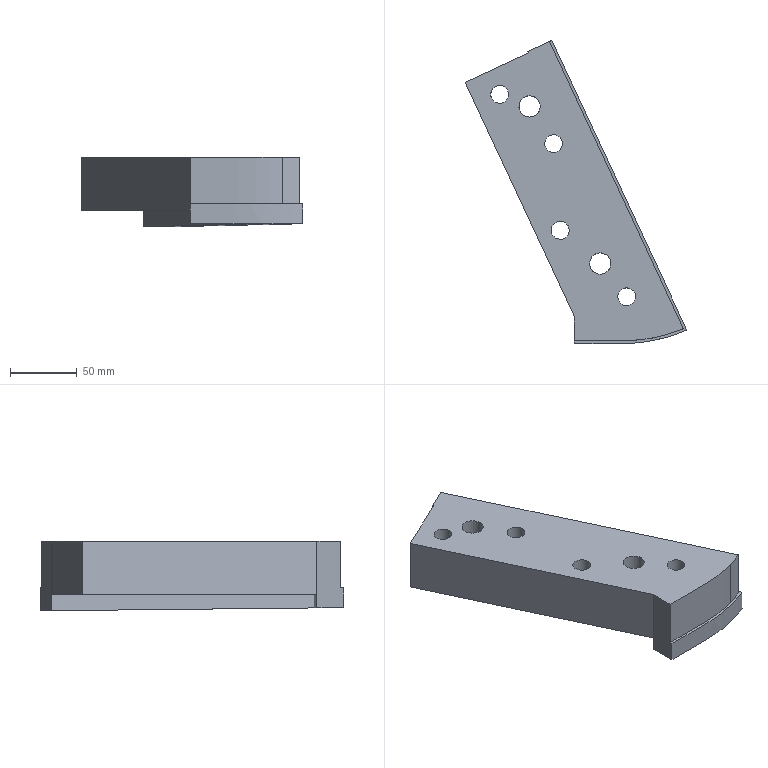Part | NX | features solid 2 | 1 solid | 32 faces | box 166.571 x 227.619 x 52.308 mm | volume 660539 mm3 | plane 17 | cylinder 10 | spline 5 | commonest cylinder face diameters 13.5 x4 19.5 x4 16 x2
STEP:
#1=CARTESIAN_POINT('',(214.067,-58.,43.));
#2=VERTEX_POINT('',#1);
#3=CARTESIAN_POINT('',(214.067,-58.,43.));
#4=VERTEX_POINT('',#3);
#5=CARTESIAN_POINT('',(192.036,-10.753,43.));
#6=DIRECTION('',(0.4226,-0.9063,0.));
#7=VECTOR('',#6,1000.);
#8=LINE('',#5,#7);
#9=EDGE_CURVE('',#2,#4,#8,.T.);
#10=ORIENTED_EDGE('',*,*,#9,.F.);
#11=CARTESIAN_POINT('',(214.067,-58.,8.));
#12=VERTEX_POINT('',#11);
#13=CARTESIAN_POINT('',(214.067,-58.,25.5));
#14=DIRECTION('',(0.,0.,-1.));
#15=VECTOR('',#14,1000.);
#16=LINE('',#13,#15);
#17=EDGE_CURVE('',#2,#12,#16,.T.);
#18=ORIENTED_EDGE('',*,*,#17,.T.);
#19=CARTESIAN_POINT('',(214.067,-58.,25.5));
#20=DIRECTION('',(0.,0.,-1.));
#21=VECTOR('',#20,1000.);
#22=LINE('',#19,#21);
#23=EDGE_CURVE('',#4,#12,#22,.T.);
#24=ORIENTED_EDGE('',*,*,#23,.F.);
#25=EDGE_LOOP('',(#10,#18,#24));
#26=FACE_BOUND('',#25,.T.);
#27=CARTESIAN_POINT('',(215.,-60.,-107.));
#28=DIRECTION('',(-0.9063,-0.4226,0.));
#29=DIRECTION('',(-0.4226,0.9063,0.));
#30=AXIS2_PLACEMENT_3D('',#27,#28,#29);
#31=PLANE('',#30);
#32=ADVANCED_FACE('',(#26),#31,.T.);
#33=CARTESIAN_POINT('',(170.586,159.137,-9.218));
#34=VERTEX_POINT('',#33);
#35=CARTESIAN_POINT('',(188.712,167.589,-9.308));
#36=VERTEX_POINT('',#35);
#37=CARTESIAN_POINT('',(155.822,152.253,-9.145));
#38=DIRECTION('',(-0.9063,-0.4226,0.004484));
#39=VECTOR('',#38,1000.);
#40=LINE('',#37,#39);
#41=EDGE_CURVE('',#34,#36,#40,.F.);
#42=ORIENTED_EDGE('',*,*,#41,.T.);
#43=CARTESIAN_POINT('',(290.127,-49.896,-7.));
#44=VERTEX_POINT('',#43);
#45=CARTESIAN_POINT('',(281.198,-30.747,-7.203));
#46=DIRECTION('',(-0.4226,0.9063,-0.009616));
#47=VECTOR('',#46,1000.);
#48=LINE('',#45,#47);
#49=EDGE_CURVE('',#36,#44,#48,.F.);
#50=ORIENTED_EDGE('',*,*,#49,.T.);
#51=CARTESIAN_POINT('',(205.676,-60.001,-6.893));
#52=VERTEX_POINT('',#51);
#53=CARTESIAN_POINT('',(205.676,-60.001,-6.893));
#54=CARTESIAN_POINT('',(212.807,-60.,-6.893));
#55=CARTESIAN_POINT('',(223.501,-59.952,-6.893));
#56=CARTESIAN_POINT('',(237.776,-60.073,-6.892));
#57=CARTESIAN_POINT('',(246.675,-59.905,-6.894));
#58=CARTESIAN_POINT('',(253.767,-59.465,-6.898));
#59=CARTESIAN_POINT('',(259.049,-58.73,-6.906));
#60=CARTESIAN_POINT('',(264.326,-57.938,-6.915));
#61=CARTESIAN_POINT('',(269.572,-56.804,-6.927));
#62=CARTESIAN_POINT('',(274.792,-55.406,-6.942));
#63=CARTESIAN_POINT('',(279.134,-54.082,-6.956));
#64=CARTESIAN_POINT('',(282.588,-52.985,-6.967));
#65=CARTESIAN_POINT('',(285.941,-51.62,-6.982));
#66=CARTESIAN_POINT('',(288.461,-50.608,-6.992));
#67=CARTESIAN_POINT('',(290.127,-49.896,-7.));
#68=B_SPLINE_CURVE_WITH_KNOTS('',3,(#53,#54,#55,#56,#57,#58,#59,#60,#61,#62,#63,#64,#65,#66,#67),.UNSPECIFIED.,.F.,.F.,(4,1,1,1,1,1,1,1,1,1,1,1,4),(-0.009286,0.01202,0.02268,0.03333,0.03866,0.04398,0.04931,0.05464,0.05996,0.06529,0.06795,0.07062,0.07594),.UNSPECIFIED.);
#69=EDGE_CURVE('',#52,#44,#68,.T.);
#70=ORIENTED_EDGE('',*,*,#69,.F.);
#71=CARTESIAN_POINT('',(205.675,-40.001,-7.105));
#72=VERTEX_POINT('',#71);
#73=CARTESIAN_POINT('',(205.675,-49.898,-7.));
#74=DIRECTION('',(0.00005303,-0.9999,0.01061));
#75=VECTOR('',#74,1000.);
#76=LINE('',#73,#75);
#77=EDGE_CURVE('',#72,#52,#76,.T.);
#78=ORIENTED_EDGE('',*,*,#77,.F.);
#79=CARTESIAN_POINT('',(205.674,-40.001,-7.105));
#80=VERTEX_POINT('',#79);
#81=CARTESIAN_POINT('',(215.618,-61.324,-6.879));
#82=DIRECTION('',(-0.4226,0.9063,-0.009616));
#83=VECTOR('',#82,1000.);
#84=LINE('',#81,#83);
#85=EDGE_CURVE('',#80,#72,#84,.F.);
#86=ORIENTED_EDGE('',*,*,#85,.F.);
#87=CARTESIAN_POINT('',(262.447,-37.86,-7.128));
#88=VERTEX_POINT('',#87);
#89=CARTESIAN_POINT('',(262.447,-37.86,-7.128));
#90=CARTESIAN_POINT('',(260.096,-38.349,-7.123));
#91=CARTESIAN_POINT('',(256.564,-38.895,-7.117));
#92=CARTESIAN_POINT('',(251.85,-39.528,-7.11));
#93=CARTESIAN_POINT('',(244.761,-40.001,-7.105));
#94=CARTESIAN_POINT('',(234.102,-40.028,-7.105));
#95=CARTESIAN_POINT('',(219.887,-39.989,-7.105));
#96=CARTESIAN_POINT('',(210.412,-40.,-7.105));
#97=CARTESIAN_POINT('',(205.674,-40.001,-7.105));
#98=B_SPLINE_CURVE_WITH_KNOTS('',3,(#89,#90,#91,#92,#93,#94,#95,#96,#97),.UNSPECIFIED.,.F.,.F.,(4,1,1,1,1,1,4),(0.,0.007102,0.01065,0.0142,0.02841,0.04261,0.05681),.UNSPECIFIED.);
#99=EDGE_CURVE('',#88,#80,#98,.T.);
#100=ORIENTED_EDGE('',*,*,#99,.F.);
#101=CARTESIAN_POINT('',(263.071,-39.199,-7.114));
#102=DIRECTION('',(-0.4226,0.9063,-0.009616));
#103=VECTOR('',#102,1000.);
#104=LINE('',#101,#103);
#105=EDGE_CURVE('',#34,#88,#104,.F.);
#106=ORIENTED_EDGE('',*,*,#105,.F.);
#107=EDGE_LOOP('',(#42,#50,#70,#78,#86,#100,#106));
#108=FACE_BOUND('',#107,.T.);
#109=CARTESIAN_POINT('',(240.127,-49.896,-7.));
#110=DIRECTION('',(0.,-0.01061,-0.9999));
#111=DIRECTION('',(0.,0.9999,-0.01061));
#112=AXIS2_PLACEMENT_3D('',#109,#110,#111);
#113=PLANE('',#112);
#114=ADVANCED_FACE('',(#108),#113,.T.);
#115=CARTESIAN_POINT('',(170.586,159.137,43.));
#116=VERTEX_POINT('',#115);
#117=CARTESIAN_POINT('',(171.008,158.231,43.));
#118=VERTEX_POINT('',#117);
#119=CARTESIAN_POINT('',(64.931,385.714,43.));
#120=DIRECTION('',(0.4226,-0.9063,0.));
#121=VECTOR('',#120,1000.);
#122=LINE('',#119,#121);
#123=EDGE_CURVE('',#116,#118,#122,.T.);
#124=ORIENTED_EDGE('',*,*,#123,.T.);
#125=CARTESIAN_POINT('',(123.556,136.103,43.));
#126=VERTEX_POINT('',#125);
#127=CARTESIAN_POINT('',(124.462,136.526,43.));
#128=DIRECTION('',(0.9063,0.4226,0.));
#129=VECTOR('',#128,1000.);
#130=LINE('',#127,#129);
#131=EDGE_CURVE('',#118,#126,#130,.F.);
#132=ORIENTED_EDGE('',*,*,#131,.T.);
#133=CARTESIAN_POINT('',(205.675,-40.001,43.));
#134=VERTEX_POINT('',#133);
#135=CARTESIAN_POINT('',(192.036,-10.753,43.));
#136=DIRECTION('',(0.4226,-0.9063,0.));
#137=VECTOR('',#136,1000.);
#138=LINE('',#135,#137);
#139=EDGE_CURVE('',#126,#134,#138,.T.);
#140=ORIENTED_EDGE('',*,*,#139,.T.);
#141=CARTESIAN_POINT('',(205.675,-58.001,43.));
#142=VERTEX_POINT('',#141);
#143=CARTESIAN_POINT('',(205.668,84.753,43.));
#144=DIRECTION('',(0.00005304,-1.,0.));
#145=VECTOR('',#144,1000.);
#146=LINE('',#143,#145);
#147=EDGE_CURVE('',#134,#142,#146,.T.);
#148=ORIENTED_EDGE('',*,*,#147,.T.);
#149=CARTESIAN_POINT('',(214.067,-58.,43.));
#150=CARTESIAN_POINT('',(211.27,-58.,43.));
#151=CARTESIAN_POINT('',(208.473,-58.,43.));
#152=CARTESIAN_POINT('',(205.675,-58.001,43.));
#153=B_SPLINE_CURVE_WITH_KNOTS('',3,(#149,#150,#151,#152),.UNSPECIFIED.,.F.,.F.,(4,4),(0.7754,0.7842),.UNSPECIFIED.);
#154=EDGE_CURVE('',#2,#142,#153,.T.);
#155=ORIENTED_EDGE('',*,*,#154,.F.);
#156=ORIENTED_EDGE('',*,*,#9,.T.);
#157=CARTESIAN_POINT('',(274.646,-53.334,43.));
#158=VERTEX_POINT('',#157);
#159=CARTESIAN_POINT('',(214.067,-58.,43.));
#160=CARTESIAN_POINT('',(219.163,-57.999,43.));
#161=CARTESIAN_POINT('',(229.355,-57.977,43.));
#162=CARTESIAN_POINT('',(242.09,-58.055,43.));
#163=CARTESIAN_POINT('',(252.284,-57.637,43.));
#164=CARTESIAN_POINT('',(259.807,-56.624,43.));
#165=CARTESIAN_POINT('',(267.291,-55.368,43.));
#166=CARTESIAN_POINT('',(272.199,-54.042,43.));
#167=CARTESIAN_POINT('',(274.646,-53.334,43.));
#168=B_SPLINE_CURVE_WITH_KNOTS('',3,(#159,#160,#161,#162,#163,#164,#165,#166,#167),.UNSPECIFIED.,.F.,.F.,(4,1,1,1,1,1,4),(-0.00294,0.01235,0.02763,0.03528,0.04292,0.05056,0.05821),.UNSPECIFIED.);
#169=EDGE_CURVE('',#4,#158,#168,.T.);
#170=ORIENTED_EDGE('',*,*,#169,.T.);
#171=CARTESIAN_POINT('',(274.646,-53.333,43.));
#172=VERTEX_POINT('',#171);
#173=CARTESIAN_POINT('',(262.155,89.442,43.));
#174=DIRECTION('',(0.08716,-0.9962,0.));
#175=VECTOR('',#174,1000.);
#176=LINE('',#173,#175);
#177=EDGE_CURVE('',#158,#172,#176,.F.);
#178=ORIENTED_EDGE('',*,*,#177,.T.);
#179=CARTESIAN_POINT('',(287.434,-48.854,43.));
#180=VERTEX_POINT('',#179);
#181=CARTESIAN_POINT('',(287.434,-48.854,43.));
#182=CARTESIAN_POINT('',(286.384,-49.285,43.));
#183=CARTESIAN_POINT('',(284.206,-50.176,43.));
#184=CARTESIAN_POINT('',(281.186,-51.367,43.));
#185=CARTESIAN_POINT('',(277.932,-52.345,43.));
#186=CARTESIAN_POINT('',(275.731,-53.015,43.));
#187=CARTESIAN_POINT('',(274.646,-53.333,43.));
#188=B_SPLINE_CURVE_WITH_KNOTS('',3,(#181,#182,#183,#184,#185,#186,#187),.UNSPECIFIED.,.F.,.F.,(4,1,1,1,4),(0.6964,0.7,0.7036,0.7072,0.7108),.UNSPECIFIED.);
#189=EDGE_CURVE('',#180,#172,#188,.T.);
#190=ORIENTED_EDGE('',*,*,#189,.F.);
#191=CARTESIAN_POINT('',(186.899,166.744,43.));
#192=VERTEX_POINT('',#191);
#193=CARTESIAN_POINT('',(81.245,393.321,43.));
#194=DIRECTION('',(-0.4226,0.9063,0.));
#195=VECTOR('',#194,1000.);
#196=LINE('',#193,#195);
#197=EDGE_CURVE('',#192,#180,#196,.F.);
#198=ORIENTED_EDGE('',*,*,#197,.F.);
#199=CARTESIAN_POINT('',(322.898,230.162,43.));
#200=DIRECTION('',(-0.9063,-0.4226,0.));
#201=VECTOR('',#200,1000.);
#202=LINE('',#199,#201);
#203=EDGE_CURVE('',#116,#192,#202,.F.);
#204=ORIENTED_EDGE('',*,*,#203,.F.);
#205=EDGE_LOOP('',(#124,#132,#140,#148,#155,#156,#170,#178,#190,#198,#204));
#206=FACE_BOUND('',#205,.T.);
#207=CARTESIAN_POINT('',(180.,118.,43.));
#208=VERTEX_POINT('',#207);
#209=CARTESIAN_POINT('',(172.,118.,43.));
#210=DIRECTION('',(0.,0.,1.));
#211=DIRECTION('',(1.,0.,0.));
#212=AXIS2_PLACEMENT_3D('',#209,#210,#211);
#213=CIRCLE('',#212,8.);
#214=EDGE_CURVE('',#208,#208,#213,.F.);
#215=ORIENTED_EDGE('',*,*,#214,.T.);
#216=EDGE_LOOP('',(#215));
#217=FACE_BOUND('',#216,.T.);
#218=CARTESIAN_POINT('',(233.,0.,43.));
#219=VERTEX_POINT('',#218);
#220=CARTESIAN_POINT('',(225.,0.,43.));
#221=DIRECTION('',(0.,0.,1.));
#222=DIRECTION('',(1.,0.,0.));
#223=AXIS2_PLACEMENT_3D('',#220,#221,#222);
#224=CIRCLE('',#223,8.);
#225=EDGE_CURVE('',#219,#219,#224,.F.);
#226=ORIENTED_EDGE('',*,*,#225,.T.);
#227=EDGE_LOOP('',(#226));
#228=FACE_BOUND('',#227,.T.);
#229=CARTESIAN_POINT('',(156.282,127.113,43.));
#230=VERTEX_POINT('',#229);
#231=CARTESIAN_POINT('',(149.532,127.113,43.));
#232=DIRECTION('',(0.,0.,1.));
#233=DIRECTION('',(1.,0.,0.));
#234=AXIS2_PLACEMENT_3D('',#231,#232,#233);
#235=CIRCLE('',#234,6.75);
#236=EDGE_CURVE('',#230,#230,#235,.F.);
#237=ORIENTED_EDGE('',*,*,#236,.T.);
#238=EDGE_LOOP('',(#237));
#239=FACE_BOUND('',#238,.T.);
#240=CARTESIAN_POINT('',(196.75,90.,43.));
#241=VERTEX_POINT('',#240);
#242=CARTESIAN_POINT('',(190.,90.,43.));
#243=DIRECTION('',(0.,0.,1.));
#244=DIRECTION('',(1.,0.,0.));
#245=AXIS2_PLACEMENT_3D('',#242,#243,#244);
#246=CIRCLE('',#245,6.75);
#247=EDGE_CURVE('',#241,#241,#246,.F.);
#248=ORIENTED_EDGE('',*,*,#247,.T.);
#249=EDGE_LOOP('',(#248));
#250=FACE_BOUND('',#249,.T.);
#251=CARTESIAN_POINT('',(201.75,25.,43.));
#252=VERTEX_POINT('',#251);
#253=CARTESIAN_POINT('',(195.,25.,43.));
#254=DIRECTION('',(0.,0.,1.));
#255=DIRECTION('',(1.,0.,0.));
#256=AXIS2_PLACEMENT_3D('',#253,#254,#255);
#257=CIRCLE('',#256,6.75);
#258=EDGE_CURVE('',#252,#252,#257,.F.);
#259=ORIENTED_EDGE('',*,*,#258,.T.);
#260=EDGE_LOOP('',(#259));
#261=FACE_BOUND('',#260,.T.);
#262=CARTESIAN_POINT('',(251.75,-25.,43.));
#263=VERTEX_POINT('',#262);
#264=CARTESIAN_POINT('',(245.,-25.,43.));
#265=DIRECTION('',(0.,0.,1.));
#266=DIRECTION('',(1.,0.,0.));
#267=AXIS2_PLACEMENT_3D('',#264,#265,#266);
#268=CIRCLE('',#267,6.75);
#269=EDGE_CURVE('',#263,#263,#268,.F.);
#270=ORIENTED_EDGE('',*,*,#269,.T.);
#271=EDGE_LOOP('',(#270));
#272=FACE_BOUND('',#271,.T.);
#273=CARTESIAN_POINT('',(383.563,100.064,43.));
#274=DIRECTION('',(0.,0.,-1.));
#275=DIRECTION('',(0.9962,0.08716,0.));
#276=AXIS2_PLACEMENT_3D('',#273,#274,#275);
#277=PLANE('',#276);
#278=ADVANCED_FACE('',(#206,#217,#228,#239,#250,#261,#272),#277,.F.);
#279=CARTESIAN_POINT('',(172.,110.,3.));
#280=VERTEX_POINT('',#279);
#281=CARTESIAN_POINT('',(172.,118.,3.));
#282=DIRECTION('',(0.,0.,-1.));
#283=DIRECTION('',(0.,-1.,0.));
#284=AXIS2_PLACEMENT_3D('',#281,#282,#283);
#285=CIRCLE('',#284,8.);
#286=EDGE_CURVE('',#280,#280,#285,.T.);
#287=ORIENTED_EDGE('',*,*,#286,.F.);
#288=EDGE_LOOP('',(#287));
#289=FACE_BOUND('',#288,.T.);
#290=CARTESIAN_POINT('',(225.,-8.,3.));
#291=VERTEX_POINT('',#290);
#292=CARTESIAN_POINT('',(225.,0.,3.));
#293=DIRECTION('',(0.,0.,-1.));
#294=DIRECTION('',(0.,-1.,0.));
#295=AXIS2_PLACEMENT_3D('',#292,#293,#294);
#296=CIRCLE('',#295,8.);
#297=EDGE_CURVE('',#291,#291,#296,.T.);
#298=ORIENTED_EDGE('',*,*,#297,.F.);
#299=EDGE_LOOP('',(#298));
#300=FACE_BOUND('',#299,.T.);
#301=CARTESIAN_POINT('',(149.532,117.363,3.));
#302=VERTEX_POINT('',#301);
#303=CARTESIAN_POINT('',(149.532,127.113,3.));
#304=DIRECTION('',(0.,0.,-1.));
#305=DIRECTION('',(0.,-1.,0.));
#306=AXIS2_PLACEMENT_3D('',#303,#304,#305);
#307=CIRCLE('',#306,9.75);
#308=EDGE_CURVE('',#302,#302,#307,.T.);
#309=ORIENTED_EDGE('',*,*,#308,.F.);
#310=EDGE_LOOP('',(#309));
#311=FACE_BOUND('',#310,.T.);
#312=CARTESIAN_POINT('',(190.,80.25,3.));
#313=VERTEX_POINT('',#312);
#314=CARTESIAN_POINT('',(190.,90.,3.));
#315=DIRECTION('',(0.,0.,-1.));
#316=DIRECTION('',(0.,-1.,0.));
#317=AXIS2_PLACEMENT_3D('',#314,#315,#316);
#318=CIRCLE('',#317,9.75);
#319=EDGE_CURVE('',#313,#313,#318,.T.);
#320=ORIENTED_EDGE('',*,*,#319,.F.);
#321=EDGE_LOOP('',(#320));
#322=FACE_BOUND('',#321,.T.);
#323=CARTESIAN_POINT('',(195.,15.25,3.));
#324=VERTEX_POINT('',#323);
#325=CARTESIAN_POINT('',(195.,25.,3.));
#326=DIRECTION('',(0.,0.,-1.));
#327=DIRECTION('',(0.,-1.,0.));
#328=AXIS2_PLACEMENT_3D('',#325,#326,#327);
#329=CIRCLE('',#328,9.75);
#330=EDGE_CURVE('',#324,#324,#329,.T.);
#331=ORIENTED_EDGE('',*,*,#330,.F.);
#332=EDGE_LOOP('',(#331));
#333=FACE_BOUND('',#332,.T.);
#334=CARTESIAN_POINT('',(245.,-34.75,3.));
#335=VERTEX_POINT('',#334);
#336=CARTESIAN_POINT('',(245.,-25.,3.));
#337=DIRECTION('',(0.,0.,-1.));
#338=DIRECTION('',(0.,-1.,0.));
#339=AXIS2_PLACEMENT_3D('',#336,#337,#338);
#340=CIRCLE('',#339,9.75);
#341=EDGE_CURVE('',#335,#335,#340,.T.);
#342=ORIENTED_EDGE('',*,*,#341,.F.);
#343=EDGE_LOOP('',(#342));
#344=FACE_BOUND('',#343,.T.);
#345=CARTESIAN_POINT('',(171.008,158.231,3.));
#346=VERTEX_POINT('',#345);
#347=CARTESIAN_POINT('',(123.556,136.103,3.));
#348=VERTEX_POINT('',#347);
#349=CARTESIAN_POINT('',(124.462,136.526,3.));
#350=DIRECTION('',(0.9063,0.4226,0.));
#351=VECTOR('',#350,1000.);
#352=LINE('',#349,#351);
#353=EDGE_CURVE('',#346,#348,#352,.F.);
#354=ORIENTED_EDGE('',*,*,#353,.F.);
#355=CARTESIAN_POINT('',(262.447,-37.86,3.));
#356=VERTEX_POINT('',#355);
#357=CARTESIAN_POINT('',(64.931,385.714,3.));
#358=DIRECTION('',(0.4226,-0.9063,0.));
#359=VECTOR('',#358,1000.);
#360=LINE('',#357,#359);
#361=EDGE_CURVE('',#346,#356,#360,.T.);
#362=ORIENTED_EDGE('',*,*,#361,.T.);
#363=CARTESIAN_POINT('',(205.674,-40.001,3.));
#364=VERTEX_POINT('',#363);
#365=CARTESIAN_POINT('',(262.447,-37.86,3.));
#366=CARTESIAN_POINT('',(260.12,-38.344,3.));
#367=CARTESIAN_POINT('',(256.612,-38.886,3.));
#368=CARTESIAN_POINT('',(251.926,-39.52,3.));
#369=CARTESIAN_POINT('',(244.85,-40.,3.));
#370=CARTESIAN_POINT('',(234.169,-40.029,3.));
#371=CARTESIAN_POINT('',(219.919,-39.989,3.));
#372=CARTESIAN_POINT('',(210.423,-40.,3.));
#373=CARTESIAN_POINT('',(205.674,-40.001,3.));
#374=B_SPLINE_CURVE_WITH_KNOTS('',3,(#365,#366,#367,#368,#369,#370,#371,#372,#373),.UNSPECIFIED.,.F.,.F.,(4,1,1,1,1,1,4),(0.07548,0.08262,0.08618,0.08975,0.104,0.1183,0.1325),.UNSPECIFIED.);
#375=EDGE_CURVE('',#364,#356,#374,.F.);
#376=ORIENTED_EDGE('',*,*,#375,.F.);
#377=CARTESIAN_POINT('',(204.661,-37.827,3.));
#378=DIRECTION('',(0.4226,-0.9063,0.));
#379=VECTOR('',#378,1000.);
#380=LINE('',#377,#379);
#381=EDGE_CURVE('',#364,#348,#380,.F.);
#382=ORIENTED_EDGE('',*,*,#381,.T.);
#383=EDGE_LOOP('',(#354,#362,#376,#382));
#384=FACE_BOUND('',#383,.T.);
#385=CARTESIAN_POINT('',(-60.069,387.73,3.));
#386=DIRECTION('',(0.,0.,-1.));
#387=DIRECTION('',(0.08716,-0.9962,0.));
#388=AXIS2_PLACEMENT_3D('',#385,#386,#387);
#389=PLANE('',#388);
#390=ADVANCED_FACE('',(#289,#300,#311,#322,#333,#344,#384),#389,.T.);
#391=CARTESIAN_POINT('',(188.712,167.589,8.));
#392=VERTEX_POINT('',#391);
#393=CARTESIAN_POINT('',(186.899,166.744,8.));
#394=VERTEX_POINT('',#393);
#395=CARTESIAN_POINT('',(85.717,119.562,8.));
#396=DIRECTION('',(0.9063,0.4226,0.));
#397=VECTOR('',#396,1000.);
#398=LINE('',#395,#397);
#399=EDGE_CURVE('',#392,#394,#398,.F.);
#400=ORIENTED_EDGE('',*,*,#399,.T.);
#401=CARTESIAN_POINT('',(287.434,-48.854,8.));
#402=VERTEX_POINT('',#401);
#403=CARTESIAN_POINT('',(81.245,393.321,8.));
#404=DIRECTION('',(-0.4226,0.9063,0.));
#405=VECTOR('',#404,1000.);
#406=LINE('',#403,#405);
#407=EDGE_CURVE('',#394,#402,#406,.F.);
#408=ORIENTED_EDGE('',*,*,#407,.T.);
#409=CARTESIAN_POINT('',(274.646,-53.333,8.));
#410=VERTEX_POINT('',#409);
#411=CARTESIAN_POINT('',(287.434,-48.854,8.));
#412=CARTESIAN_POINT('',(286.384,-49.285,8.));
#413=CARTESIAN_POINT('',(284.206,-50.176,8.));
#414=CARTESIAN_POINT('',(281.186,-51.367,8.));
#415=CARTESIAN_POINT('',(277.932,-52.345,8.));
#416=CARTESIAN_POINT('',(275.731,-53.015,8.));
#417=CARTESIAN_POINT('',(274.646,-53.333,8.));
#418=B_SPLINE_CURVE_WITH_KNOTS('',3,(#411,#412,#413,#414,#415,#416,#417),.UNSPECIFIED.,.F.,.F.,(4,1,1,1,4),(0.6964,0.7,0.7036,0.7072,0.7108),.UNSPECIFIED.);
#419=EDGE_CURVE('',#402,#410,#418,.T.);
#420=ORIENTED_EDGE('',*,*,#419,.T.);
#421=CARTESIAN_POINT('',(274.646,-53.334,8.));
#422=VERTEX_POINT('',#421);
#423=CARTESIAN_POINT('',(274.772,-54.771,8.));
#424=DIRECTION('',(-0.08716,0.9962,0.));
#425=VECTOR('',#424,1000.);
#426=LINE('',#423,#425);
#427=EDGE_CURVE('',#422,#410,#426,.T.);
#428=ORIENTED_EDGE('',*,*,#427,.F.);
#429=CARTESIAN_POINT('',(214.067,-58.,8.));
#430=CARTESIAN_POINT('',(219.163,-57.999,8.));
#431=CARTESIAN_POINT('',(229.355,-57.977,8.));
#432=CARTESIAN_POINT('',(242.089,-58.055,8.));
#433=CARTESIAN_POINT('',(252.284,-57.637,8.));
#434=CARTESIAN_POINT('',(259.807,-56.624,8.));
#435=CARTESIAN_POINT('',(267.292,-55.368,8.));
#436=CARTESIAN_POINT('',(272.2,-54.042,8.));
#437=CARTESIAN_POINT('',(274.646,-53.334,8.));
#438=B_SPLINE_CURVE_WITH_KNOTS('',3,(#429,#430,#431,#432,#433,#434,#435,#436,#437),.UNSPECIFIED.,.F.,.F.,(4,1,1,1,1,1,4),(-0.002765,0.01252,0.02781,0.03545,0.04309,0.05074,0.05838),.UNSPECIFIED.);
#439=EDGE_CURVE('',#12,#422,#438,.T.);
#440=ORIENTED_EDGE('',*,*,#439,.F.);
#441=CARTESIAN_POINT('',(205.675,-58.001,8.));
#442=VERTEX_POINT('',#441);
#443=CARTESIAN_POINT('',(214.067,-58.,8.));
#444=CARTESIAN_POINT('',(211.27,-58.,8.));
#445=CARTESIAN_POINT('',(208.473,-58.,8.));
#446=CARTESIAN_POINT('',(205.675,-58.001,8.));
#447=B_SPLINE_CURVE_WITH_KNOTS('',3,(#443,#444,#445,#446),.UNSPECIFIED.,.F.,.F.,(4,4),(0.7754,0.7842),.UNSPECIFIED.);
#448=EDGE_CURVE('',#12,#442,#447,.T.);
#449=ORIENTED_EDGE('',*,*,#448,.T.);
#450=CARTESIAN_POINT('',(205.676,-60.001,8.));
#451=VERTEX_POINT('',#450);
#452=CARTESIAN_POINT('',(205.65,429.974,8.));
#453=DIRECTION('',(-0.00005304,1.,0.));
#454=VECTOR('',#453,1000.);
#455=LINE('',#452,#454);
#456=EDGE_CURVE('',#442,#451,#455,.F.);
#457=ORIENTED_EDGE('',*,*,#456,.T.);
#458=CARTESIAN_POINT('',(215.,-60.,8.));
#459=VERTEX_POINT('',#458);
#460=CARTESIAN_POINT('',(205.676,-60.001,8.));
#461=CARTESIAN_POINT('',(206.425,-60.001,8.));
#462=CARTESIAN_POINT('',(207.882,-60.001,8.));
#463=CARTESIAN_POINT('',(211.055,-60.,8.));
#464=CARTESIAN_POINT('',(213.431,-60.,8.));
#465=CARTESIAN_POINT('',(215.,-60.,8.));
#466=B_SPLINE_CURVE_WITH_KNOTS('',3,(#460,#461,#462,#463,#464,#465),.UNSPECIFIED.,.F.,.F.,(4,1,1,4),(0.2156,0.2181,0.2206,0.2255),.UNSPECIFIED.);
#467=EDGE_CURVE('',#459,#451,#466,.F.);
#468=ORIENTED_EDGE('',*,*,#467,.F.);
#469=CARTESIAN_POINT('',(274.824,-55.364,8.));
#470=VERTEX_POINT('',#469);
#471=CARTESIAN_POINT('',(274.824,-55.364,8.));
#472=CARTESIAN_POINT('',(272.371,-56.074,8.));
#473=CARTESIAN_POINT('',(267.457,-57.375,8.));
#474=CARTESIAN_POINT('',(260.029,-58.61,8.));
#475=CARTESIAN_POINT('',(252.585,-59.618,8.));
#476=CARTESIAN_POINT('',(245.086,-59.927,8.));
#477=CARTESIAN_POINT('',(237.573,-60.058,8.));
#478=CARTESIAN_POINT('',(227.535,-59.965,8.));
#479=CARTESIAN_POINT('',(220.015,-59.999,8.));
#480=CARTESIAN_POINT('',(215.,-60.,8.));
#481=B_SPLINE_CURVE_WITH_KNOTS('',3,(#471,#472,#473,#474,#475,#476,#477,#478,#479,#480),.UNSPECIFIED.,.F.,.F.,(4,1,1,1,1,1,1,4),(0.,0.0075,0.015,0.0225,0.03,0.0375,0.045,0.06),.UNSPECIFIED.);
#482=EDGE_CURVE('',#470,#459,#481,.T.);
#483=ORIENTED_EDGE('',*,*,#482,.F.);
#484=CARTESIAN_POINT('',(290.127,-49.896,8.));
#485=VERTEX_POINT('',#484);
#486=CARTESIAN_POINT('',(274.824,-55.364,8.));
#487=CARTESIAN_POINT('',(275.15,-55.27,8.));
#488=CARTESIAN_POINT('',(275.64,-55.126,8.));
#489=CARTESIAN_POINT('',(276.722,-54.802,8.));
#490=CARTESIAN_POINT('',(277.734,-54.497,8.));
#491=CARTESIAN_POINT('',(278.338,-54.314,8.));
#492=CARTESIAN_POINT('',(278.669,-54.213,8.));
#493=CARTESIAN_POINT('',(279.265,-54.031,8.));
#494=CARTESIAN_POINT('',(279.745,-53.883,8.));
#495=CARTESIAN_POINT('',(280.187,-53.745,8.));
#496=CARTESIAN_POINT('',(280.814,-53.548,8.));
#497=CARTESIAN_POINT('',(281.532,-53.313,8.));
#498=CARTESIAN_POINT('',(282.084,-53.126,8.));
#499=CARTESIAN_POINT('',(282.731,-52.898,8.));
#500=CARTESIAN_POINT('',(283.309,-52.682,8.));
#501=CARTESIAN_POINT('',(283.991,-52.414,8.));
#502=CARTESIAN_POINT('',(284.387,-52.255,8.));
#503=CARTESIAN_POINT('',(284.936,-52.031,8.));
#504=CARTESIAN_POINT('',(285.292,-51.886,8.));
#505=CARTESIAN_POINT('',(285.642,-51.742,8.));
#506=CARTESIAN_POINT('',(285.81,-51.674,8.));
#507=CARTESIAN_POINT('',(286.171,-51.527,8.));
#508=CARTESIAN_POINT('',(286.882,-51.238,8.));
#509=CARTESIAN_POINT('',(287.218,-51.102,8.));
#510=CARTESIAN_POINT('',(287.366,-51.042,8.));
#511=CARTESIAN_POINT('',(287.365,-51.042,8.));
#512=CARTESIAN_POINT('',(287.562,-50.962,8.));
#513=CARTESIAN_POINT('',(287.858,-50.842,8.));
#514=CARTESIAN_POINT('',(288.274,-50.672,8.));
#515=CARTESIAN_POINT('',(288.732,-50.483,8.));
#516=CARTESIAN_POINT('',(289.243,-50.271,8.));
#517=CARTESIAN_POINT('',(289.804,-50.034,8.));
#518=CARTESIAN_POINT('',(290.127,-49.896,8.));
#519=B_SPLINE_CURVE_WITH_KNOTS('',3,(#486,#487,#488,#489,#490,#491,#492,#493,#494,#495,#496,#497,#498,#499,#500,#501,#502,#503,#504,#505,#506,#507,#508,#509,#510,#511,#512,#513,#514,#515,#516,#517,#518),.UNSPECIFIED.,.F.,.F.,(4,1,1,1,1,1,1,1,1,1,1,1,1,1,1,1,1,1,1,1,1,1,1,1,1,1,1,1,1,1,4),(0.2888,0.2898,0.2909,0.292,0.2925,0.293,0.2936,0.2941,0.2946,0.2952,0.2962,0.2967,0.2973,0.2983,0.2989,0.2994,0.2999,0.3005,0.3007,0.301,0.3015,0.3021,0.3023,0.3026,0.3027,0.3029,0.3031,0.3036,0.3042,0.3047,0.3058),.UNSPECIFIED.);
#520=EDGE_CURVE('',#485,#470,#519,.F.);
#521=ORIENTED_EDGE('',*,*,#520,.F.);
#522=CARTESIAN_POINT('',(178.495,189.499,8.));
#523=DIRECTION('',(-0.4226,0.9063,0.));
#524=VECTOR('',#523,1000.);
#525=LINE('',#522,#524);
#526=EDGE_CURVE('',#392,#485,#525,.F.);
#527=ORIENTED_EDGE('',*,*,#526,.F.);
#528=EDGE_LOOP('',(#400,#408,#420,#428,#440,#449,#457,#468,#483,#521,#527));
#529=FACE_BOUND('',#528,.T.);
#530=CARTESIAN_POINT('',(-40.145,389.473,8.));
#531=DIRECTION('',(0.,0.,1.));
#532=DIRECTION('',(0.08716,-0.9962,0.));
#533=AXIS2_PLACEMENT_3D('',#530,#531,#532);
#534=PLANE('',#533);
#535=ADVANCED_FACE('',(#529),#534,.T.);
#536=CARTESIAN_POINT('',(123.556,136.103,-107.));
#537=DIRECTION('',(0.,0.,1.));
#538=VECTOR('',#537,1000.);
#539=LINE('',#536,#538);
#540=EDGE_CURVE('',#348,#126,#539,.T.);
#541=ORIENTED_EDGE('',*,*,#540,.F.);
#542=ORIENTED_EDGE('',*,*,#381,.F.);
#543=CARTESIAN_POINT('',(205.674,-40.001,-4.5));
#544=DIRECTION('',(0.,0.,-1.));
#545=VECTOR('',#544,1000.);
#546=LINE('',#543,#545);
#547=EDGE_CURVE('',#364,#80,#546,.T.);
#548=ORIENTED_EDGE('',*,*,#547,.T.);
#549=ORIENTED_EDGE('',*,*,#85,.T.);
#550=CARTESIAN_POINT('',(205.675,-40.001,-107.));
#551=DIRECTION('',(0.,0.,1.));
#552=VECTOR('',#551,1000.);
#553=LINE('',#550,#552);
#554=EDGE_CURVE('',#72,#134,#553,.T.);
#555=ORIENTED_EDGE('',*,*,#554,.T.);
#556=ORIENTED_EDGE('',*,*,#139,.F.);
#557=EDGE_LOOP('',(#541,#542,#548,#549,#555,#556));
#558=FACE_BOUND('',#557,.T.);
#559=CARTESIAN_POINT('',(215.,-60.,-107.));
#560=DIRECTION('',(-0.9063,-0.4226,0.));
#561=DIRECTION('',(-0.4226,0.9063,0.));
#562=AXIS2_PLACEMENT_3D('',#559,#560,#561);
#563=PLANE('',#562);
#564=ADVANCED_FACE('',(#558),#563,.T.);
#565=CARTESIAN_POINT('',(188.712,167.589,-105.));
#566=DIRECTION('',(0.,0.,1.));
#567=VECTOR('',#566,1000.);
#568=LINE('',#565,#567);
#569=EDGE_CURVE('',#36,#392,#568,.T.);
#570=ORIENTED_EDGE('',*,*,#569,.T.);
#571=ORIENTED_EDGE('',*,*,#526,.T.);
#572=CARTESIAN_POINT('',(290.127,-49.896,0.5));
#573=DIRECTION('',(0.,0.,-1.));
#574=VECTOR('',#573,1000.);
#575=LINE('',#572,#574);
#576=EDGE_CURVE('',#485,#44,#575,.T.);
#577=ORIENTED_EDGE('',*,*,#576,.T.);
#578=ORIENTED_EDGE('',*,*,#49,.F.);
#579=EDGE_LOOP('',(#570,#571,#577,#578));
#580=FACE_BOUND('',#579,.T.);
#581=CARTESIAN_POINT('',(290.14,-49.924,-105.));
#582=DIRECTION('',(-0.9063,-0.4226,0.));
#583=DIRECTION('',(-0.4226,0.9063,0.));
#584=AXIS2_PLACEMENT_3D('',#581,#582,#583);
#585=PLANE('',#584);
#586=ADVANCED_FACE('',(#580),#585,.F.);
#587=ORIENTED_EDGE('',*,*,#105,.T.);
#588=CARTESIAN_POINT('',(262.447,-37.86,3.));
#589=DIRECTION('',(0.,0.,-1.));
#590=VECTOR('',#589,1000.);
#591=LINE('',#588,#590);
#592=EDGE_CURVE('',#88,#356,#591,.F.);
#593=ORIENTED_EDGE('',*,*,#592,.T.);
#594=ORIENTED_EDGE('',*,*,#361,.F.);
#595=CARTESIAN_POINT('',(171.008,158.231,3.));
#596=DIRECTION('',(0.,0.,-1.));
#597=VECTOR('',#596,1000.);
#598=LINE('',#595,#597);
#599=EDGE_CURVE('',#346,#118,#598,.F.);
#600=ORIENTED_EDGE('',*,*,#599,.T.);
#601=ORIENTED_EDGE('',*,*,#123,.F.);
#602=CARTESIAN_POINT('',(170.586,159.137,3.));
#603=DIRECTION('',(0.,0.,1.));
#604=VECTOR('',#603,1000.);
#605=LINE('',#602,#604);
#606=EDGE_CURVE('',#34,#116,#605,.T.);
#607=ORIENTED_EDGE('',*,*,#606,.F.);
#608=EDGE_LOOP('',(#587,#593,#594,#600,#601,#607));
#609=FACE_BOUND('',#608,.T.);
#610=CARTESIAN_POINT('',(64.931,385.714,3.));
#611=DIRECTION('',(-0.9063,-0.4226,0.));
#612=DIRECTION('',(-0.4226,0.9063,0.));
#613=AXIS2_PLACEMENT_3D('',#610,#611,#612);
#614=PLANE('',#613);
#615=ADVANCED_FACE('',(#609),#614,.T.);
#616=CARTESIAN_POINT('',(186.899,166.744,43.));
#617=DIRECTION('',(0.,0.,1.));
#618=VECTOR('',#617,1000.);
#619=LINE('',#616,#618);
#620=EDGE_CURVE('',#394,#192,#619,.T.);
#621=ORIENTED_EDGE('',*,*,#620,.T.);
#622=ORIENTED_EDGE('',*,*,#197,.T.);
#623=CARTESIAN_POINT('',(287.434,-48.854,25.5));
#624=DIRECTION('',(0.,0.,-1.));
#625=VECTOR('',#624,1000.);
#626=LINE('',#623,#625);
#627=EDGE_CURVE('',#180,#402,#626,.T.);
#628=ORIENTED_EDGE('',*,*,#627,.T.);
#629=ORIENTED_EDGE('',*,*,#407,.F.);
#630=EDGE_LOOP('',(#621,#622,#628,#629));
#631=FACE_BOUND('',#630,.T.);
#632=CARTESIAN_POINT('',(81.245,393.321,43.));
#633=DIRECTION('',(-0.9063,-0.4226,0.));
#634=DIRECTION('',(-0.4226,0.9063,0.));
#635=AXIS2_PLACEMENT_3D('',#632,#633,#634);
#636=PLANE('',#635);
#637=ADVANCED_FACE('',(#631),#636,.F.);
#638=CARTESIAN_POINT('',(274.646,-53.333,25.5));
#639=DIRECTION('',(0.,0.,-1.));
#640=VECTOR('',#639,1000.);
#641=LINE('',#638,#640);
#642=EDGE_CURVE('',#410,#172,#641,.F.);
#643=ORIENTED_EDGE('',*,*,#642,.T.);
#644=ORIENTED_EDGE('',*,*,#177,.F.);
#645=CARTESIAN_POINT('',(274.646,-53.334,33.));
#646=DIRECTION('',(0.,0.,-1.));
#647=VECTOR('',#646,1000.);
#648=LINE('',#645,#647);
#649=EDGE_CURVE('',#158,#422,#648,.T.);
#650=ORIENTED_EDGE('',*,*,#649,.T.);
#651=ORIENTED_EDGE('',*,*,#427,.T.);
#652=EDGE_LOOP('',(#643,#644,#650,#651));
#653=FACE_BOUND('',#652,.T.);
#654=CARTESIAN_POINT('',(274.772,-54.771,-5.));
#655=DIRECTION('',(-0.9962,-0.08716,0.));
#656=DIRECTION('',(0.,0.,-1.));
#657=AXIS2_PLACEMENT_3D('',#654,#655,#656);
#658=PLANE('',#657);
#659=ADVANCED_FACE('',(#653),#658,.F.);
#660=ORIENTED_EDGE('',*,*,#482,.T.);
#661=ORIENTED_EDGE('',*,*,#467,.T.);
#662=CARTESIAN_POINT('',(205.676,-60.001,0.5));
#663=DIRECTION('',(0.,0.,-1.));
#664=VECTOR('',#663,1000.);
#665=LINE('',#662,#664);
#666=EDGE_CURVE('',#451,#52,#665,.T.);
#667=ORIENTED_EDGE('',*,*,#666,.T.);
#668=ORIENTED_EDGE('',*,*,#69,.T.);
#669=ORIENTED_EDGE('',*,*,#576,.F.);
#670=ORIENTED_EDGE('',*,*,#520,.T.);
#671=EDGE_LOOP('',(#660,#661,#667,#668,#669,#670));
#672=FACE_BOUND('',#671,.T.);
#673=CARTESIAN_POINT('',(290.127,-49.896,8.));
#674=CARTESIAN_POINT('',(290.127,-49.896,-7.09));
#675=CARTESIAN_POINT('',(288.482,-50.599,8.));
#676=CARTESIAN_POINT('',(288.482,-50.599,-7.09));
#677=CARTESIAN_POINT('',(285.992,-51.597,8.));
#678=CARTESIAN_POINT('',(285.992,-51.597,-7.09));
#679=CARTESIAN_POINT('',(282.68,-52.951,8.));
#680=CARTESIAN_POINT('',(282.68,-52.951,-7.09));
#681=CARTESIAN_POINT('',(279.274,-54.041,8.));
#682=CARTESIAN_POINT('',(279.274,-54.041,-7.09));
#683=CARTESIAN_POINT('',(274.995,-55.345,8.));
#684=CARTESIAN_POINT('',(274.995,-55.345,-7.09));
#685=CARTESIAN_POINT('',(269.814,-56.742,8.));
#686=CARTESIAN_POINT('',(269.814,-56.742,-7.09));
#687=CARTESIAN_POINT('',(264.573,-57.897,8.));
#688=CARTESIAN_POINT('',(264.573,-57.897,-7.09));
#689=CARTESIAN_POINT('',(259.265,-58.696,8.));
#690=CARTESIAN_POINT('',(259.265,-58.696,-7.09));
#691=CARTESIAN_POINT('',(253.953,-59.449,8.));
#692=CARTESIAN_POINT('',(253.953,-59.449,-7.09));
#693=CARTESIAN_POINT('',(246.809,-59.903,8.));
#694=CARTESIAN_POINT('',(246.809,-59.903,-7.09));
#695=CARTESIAN_POINT('',(237.869,-60.073,8.));
#696=CARTESIAN_POINT('',(237.869,-60.073,-7.09));
#697=CARTESIAN_POINT('',(223.559,-59.952,8.));
#698=CARTESIAN_POINT('',(223.559,-59.952,-7.09));
#699=CARTESIAN_POINT('',(212.829,-60.,8.));
#700=CARTESIAN_POINT('',(212.829,-60.,-7.09));
#701=CARTESIAN_POINT('',(205.676,-60.001,8.));
#702=CARTESIAN_POINT('',(205.676,-60.001,-7.09));
#703=B_SPLINE_SURFACE_WITH_KNOTS('',3,1,((#673,#674),(#675,#676),(#677,#678),(#679,#680),(#681,#682),(#683,#684),(#685,#686),(#687,#688),(#689,#690),(#691,#692),(#693,#694),(#695,#696),(#697,#698),(#699,#700),(#701,#702)),.SURF_OF_LINEAR_EXTRUSION.,.F.,.F.,.F.,(4,1,1,1,1,1,1,1,1,1,1,1,4),(2,2),(0.6876,0.6933,0.6962,0.6991,0.7048,0.7106,0.7163,0.7221,0.7278,0.7336,0.7451,0.7566,0.7796),(0.,1.),.UNSPECIFIED.);
#704=ADVANCED_FACE('',(#672),#703,.T.);
#705=ORIENTED_EDGE('',*,*,#439,.T.);
#706=ORIENTED_EDGE('',*,*,#649,.F.);
#707=ORIENTED_EDGE('',*,*,#169,.F.);
#708=ORIENTED_EDGE('',*,*,#23,.T.);
#709=EDGE_LOOP('',(#705,#706,#707,#708));
#710=FACE_BOUND('',#709,.T.);
#711=CARTESIAN_POINT('',(213.698,-58.,43.));
#712=CARTESIAN_POINT('',(213.698,-58.,8.));
#713=CARTESIAN_POINT('',(218.855,-57.999,43.));
#714=CARTESIAN_POINT('',(218.855,-57.999,8.));
#715=CARTESIAN_POINT('',(226.58,-57.966,43.));
#716=CARTESIAN_POINT('',(226.58,-57.966,8.));
#717=CARTESIAN_POINT('',(236.929,-58.052,43.));
#718=CARTESIAN_POINT('',(236.929,-58.052,8.));
#719=CARTESIAN_POINT('',(244.569,-57.952,43.));
#720=CARTESIAN_POINT('',(244.569,-57.952,8.));
#721=CARTESIAN_POINT('',(250.947,-57.674,43.));
#722=CARTESIAN_POINT('',(250.947,-57.674,8.));
#723=CARTESIAN_POINT('',(255.911,-57.179,43.));
#724=CARTESIAN_POINT('',(255.911,-57.179,8.));
#725=CARTESIAN_POINT('',(259.694,-56.598,43.));
#726=CARTESIAN_POINT('',(259.694,-56.598,8.));
#727=CARTESIAN_POINT('',(263.498,-56.023,43.));
#728=CARTESIAN_POINT('',(263.498,-56.023,8.));
#729=CARTESIAN_POINT('',(267.174,-55.299,43.));
#730=CARTESIAN_POINT('',(267.174,-55.299,8.));
#731=CARTESIAN_POINT('',(270.927,-54.37,43.));
#732=CARTESIAN_POINT('',(270.927,-54.37,8.));
#733=CARTESIAN_POINT('',(273.386,-53.698,43.));
#734=CARTESIAN_POINT('',(273.386,-53.698,8.));
#735=CARTESIAN_POINT('',(274.646,-53.334,43.));
#736=CARTESIAN_POINT('',(274.646,-53.334,8.));
#737=B_SPLINE_SURFACE_WITH_KNOTS('',3,1,((#711,#712),(#713,#714),(#715,#716),(#717,#718),(#719,#720),(#721,#722),(#723,#724),(#725,#726),(#727,#728),(#729,#730),(#731,#732),(#733,#734),(#735,#736)),.SURF_OF_LINEAR_EXTRUSION.,.F.,.F.,.F.,(4,1,1,1,1,1,1,1,1,1,4),(2,2),(-0.05687,0.209,0.342,0.4749,0.6078,0.6743,0.7408,0.8072,0.8737,0.9402,1.007),(0.,1.),.UNSPECIFIED.);
#738=ADVANCED_FACE('',(#710),#737,.F.);
#739=ORIENTED_EDGE('',*,*,#99,.T.);
#740=ORIENTED_EDGE('',*,*,#547,.F.);
#741=ORIENTED_EDGE('',*,*,#375,.T.);
#742=ORIENTED_EDGE('',*,*,#592,.F.);
#743=EDGE_LOOP('',(#739,#740,#741,#742));
#744=FACE_BOUND('',#743,.T.);
#745=CARTESIAN_POINT('',(262.447,-37.86,3.));
#746=CARTESIAN_POINT('',(262.447,-37.86,-7.188));
#747=CARTESIAN_POINT('',(260.125,-38.343,3.));
#748=CARTESIAN_POINT('',(260.125,-38.343,-7.188));
#749=CARTESIAN_POINT('',(256.608,-38.887,3.));
#750=CARTESIAN_POINT('',(256.608,-38.887,-7.188));
#751=CARTESIAN_POINT('',(251.907,-39.523,3.));
#752=CARTESIAN_POINT('',(251.907,-39.523,-7.188));
#753=CARTESIAN_POINT('',(244.805,-40.001,3.));
#754=CARTESIAN_POINT('',(244.805,-40.001,-7.188));
#755=CARTESIAN_POINT('',(234.131,-40.028,3.));
#756=CARTESIAN_POINT('',(234.131,-40.028,-7.188));
#757=CARTESIAN_POINT('',(219.903,-39.989,3.));
#758=CARTESIAN_POINT('',(219.903,-39.989,-7.188));
#759=CARTESIAN_POINT('',(210.417,-40.,3.));
#760=CARTESIAN_POINT('',(210.417,-40.,-7.188));
#761=CARTESIAN_POINT('',(205.674,-40.001,3.));
#762=CARTESIAN_POINT('',(205.674,-40.001,-7.188));
#763=B_SPLINE_SURFACE_WITH_KNOTS('',3,1,((#745,#746),(#747,#748),(#749,#750),(#751,#752),(#753,#754),(#755,#756),(#757,#758),(#759,#760),(#761,#762)),.SURF_OF_LINEAR_EXTRUSION.,.F.,.F.,.F.,(4,1,1,1,1,1,4),(2,2),(0.8194,0.8399,0.8502,0.8605,0.9015,0.9426,0.9836),(0.,1.),.UNSPECIFIED.);
#764=ADVANCED_FACE('',(#744),#763,.F.);
#765=ORIENTED_EDGE('',*,*,#189,.T.);
#766=ORIENTED_EDGE('',*,*,#642,.F.);
#767=ORIENTED_EDGE('',*,*,#419,.F.);
#768=ORIENTED_EDGE('',*,*,#627,.F.);
#769=EDGE_LOOP('',(#765,#766,#767,#768));
#770=FACE_BOUND('',#769,.T.);
#771=CARTESIAN_POINT('',(287.434,-48.854,43.));
#772=CARTESIAN_POINT('',(287.434,-48.854,8.));
#773=CARTESIAN_POINT('',(286.384,-49.285,43.));
#774=CARTESIAN_POINT('',(286.384,-49.285,8.));
#775=CARTESIAN_POINT('',(284.206,-50.176,43.));
#776=CARTESIAN_POINT('',(284.206,-50.176,8.));
#777=CARTESIAN_POINT('',(281.186,-51.367,43.));
#778=CARTESIAN_POINT('',(281.186,-51.367,8.));
#779=CARTESIAN_POINT('',(277.932,-52.345,43.));
#780=CARTESIAN_POINT('',(277.932,-52.345,8.));
#781=CARTESIAN_POINT('',(275.731,-53.015,43.));
#782=CARTESIAN_POINT('',(275.731,-53.015,8.));
#783=CARTESIAN_POINT('',(274.646,-53.333,43.));
#784=CARTESIAN_POINT('',(274.646,-53.333,8.));
#785=B_SPLINE_SURFACE_WITH_KNOTS('',3,1,((#771,#772),(#773,#774),(#775,#776),(#777,#778),(#779,#780),(#781,#782),(#783,#784)),.SURF_OF_LINEAR_EXTRUSION.,.F.,.F.,.F.,(4,1,1,1,4),(2,2),(0.6964,0.7,0.7036,0.7072,0.7108),(0.,1.),.UNSPECIFIED.);
#786=ADVANCED_FACE('',(#770),#785,.T.);
#787=ORIENTED_EDGE('',*,*,#606,.T.);
#788=ORIENTED_EDGE('',*,*,#203,.T.);
#789=ORIENTED_EDGE('',*,*,#620,.F.);
#790=ORIENTED_EDGE('',*,*,#399,.F.);
#791=ORIENTED_EDGE('',*,*,#569,.F.);
#792=ORIENTED_EDGE('',*,*,#41,.F.);
#793=EDGE_LOOP('',(#787,#788,#789,#790,#791,#792));
#794=FACE_BOUND('',#793,.T.);
#795=CARTESIAN_POINT('',(155.922,152.3,15.5));
#796=DIRECTION('',(-0.4226,0.9063,0.));
#797=DIRECTION('',(0.9063,0.4226,0.));
#798=AXIS2_PLACEMENT_3D('',#795,#796,#797);
#799=PLANE('',#798);
#800=ADVANCED_FACE('',(#794),#799,.T.);
#801=ORIENTED_EDGE('',*,*,#269,.F.);
#802=EDGE_LOOP('',(#801));
#803=FACE_BOUND('',#802,.T.);
#804=CARTESIAN_POINT('',(245.,-31.75,28.));
#805=VERTEX_POINT('',#804);
#806=CARTESIAN_POINT('',(245.,-25.,28.));
#807=DIRECTION('',(0.,0.,-1.));
#808=DIRECTION('',(0.,-1.,0.));
#809=AXIS2_PLACEMENT_3D('',#806,#807,#808);
#810=CIRCLE('',#809,6.75);
#811=EDGE_CURVE('',#805,#805,#810,.T.);
#812=ORIENTED_EDGE('',*,*,#811,.T.);
#813=EDGE_LOOP('',(#812));
#814=FACE_BOUND('',#813,.T.);
#815=CARTESIAN_POINT('',(245.,-25.,53.));
#816=DIRECTION('',(0.,0.,1.));
#817=DIRECTION('',(0.,-1.,0.));
#818=AXIS2_PLACEMENT_3D('',#815,#816,#817);
#819=CYLINDRICAL_SURFACE('',#818,6.75);
#820=ADVANCED_FACE('',(#803,#814),#819,.F.);
#821=ORIENTED_EDGE('',*,*,#811,.F.);
#822=EDGE_LOOP('',(#821));
#823=FACE_BOUND('',#822,.T.);
#824=CARTESIAN_POINT('',(245.,-34.75,28.));
#825=VERTEX_POINT('',#824);
#826=CARTESIAN_POINT('',(245.,-25.,28.));
#827=DIRECTION('',(0.,0.,-1.));
#828=DIRECTION('',(0.,-1.,0.));
#829=AXIS2_PLACEMENT_3D('',#826,#827,#828);
#830=CIRCLE('',#829,9.75);
#831=EDGE_CURVE('',#825,#825,#830,.T.);
#832=ORIENTED_EDGE('',*,*,#831,.T.);
#833=EDGE_LOOP('',(#832));
#834=FACE_BOUND('',#833,.T.);
#835=CARTESIAN_POINT('',(245.,-25.,28.));
#836=DIRECTION('',(0.,0.,1.));
#837=DIRECTION('',(0.,-1.,0.));
#838=AXIS2_PLACEMENT_3D('',#835,#836,#837);
#839=PLANE('',#838);
#840=ADVANCED_FACE('',(#823,#834),#839,.F.);
#841=ORIENTED_EDGE('',*,*,#831,.F.);
#842=EDGE_LOOP('',(#841));
#843=FACE_BOUND('',#842,.T.);
#844=ORIENTED_EDGE('',*,*,#341,.T.);
#845=EDGE_LOOP('',(#844));
#846=FACE_BOUND('',#845,.T.);
#847=CARTESIAN_POINT('',(245.,-25.,3.));
#848=DIRECTION('',(0.,0.,1.));
#849=DIRECTION('',(0.,-1.,0.));
#850=AXIS2_PLACEMENT_3D('',#847,#848,#849);
#851=CYLINDRICAL_SURFACE('',#850,9.75);
#852=ADVANCED_FACE('',(#843,#846),#851,.F.);
#853=ORIENTED_EDGE('',*,*,#258,.F.);
#854=EDGE_LOOP('',(#853));
#855=FACE_BOUND('',#854,.T.);
#856=CARTESIAN_POINT('',(195.,18.25,28.));
#857=VERTEX_POINT('',#856);
#858=CARTESIAN_POINT('',(195.,25.,28.));
#859=DIRECTION('',(0.,0.,-1.));
#860=DIRECTION('',(0.,-1.,0.));
#861=AXIS2_PLACEMENT_3D('',#858,#859,#860);
#862=CIRCLE('',#861,6.75);
#863=EDGE_CURVE('',#857,#857,#862,.T.);
#864=ORIENTED_EDGE('',*,*,#863,.T.);
#865=EDGE_LOOP('',(#864));
#866=FACE_BOUND('',#865,.T.);
#867=CARTESIAN_POINT('',(195.,25.,53.));
#868=DIRECTION('',(0.,0.,1.));
#869=DIRECTION('',(0.,-1.,0.));
#870=AXIS2_PLACEMENT_3D('',#867,#868,#869);
#871=CYLINDRICAL_SURFACE('',#870,6.75);
#872=ADVANCED_FACE('',(#855,#866),#871,.F.);
#873=ORIENTED_EDGE('',*,*,#863,.F.);
#874=EDGE_LOOP('',(#873));
#875=FACE_BOUND('',#874,.T.);
#876=CARTESIAN_POINT('',(195.,15.25,28.));
#877=VERTEX_POINT('',#876);
#878=CARTESIAN_POINT('',(195.,25.,28.));
#879=DIRECTION('',(0.,0.,-1.));
#880=DIRECTION('',(0.,-1.,0.));
#881=AXIS2_PLACEMENT_3D('',#878,#879,#880);
#882=CIRCLE('',#881,9.75);
#883=EDGE_CURVE('',#877,#877,#882,.T.);
#884=ORIENTED_EDGE('',*,*,#883,.T.);
#885=EDGE_LOOP('',(#884));
#886=FACE_BOUND('',#885,.T.);
#887=CARTESIAN_POINT('',(195.,25.,28.));
#888=DIRECTION('',(0.,0.,1.));
#889=DIRECTION('',(0.,-1.,0.));
#890=AXIS2_PLACEMENT_3D('',#887,#888,#889);
#891=PLANE('',#890);
#892=ADVANCED_FACE('',(#875,#886),#891,.F.);
#893=ORIENTED_EDGE('',*,*,#883,.F.);
#894=EDGE_LOOP('',(#893));
#895=FACE_BOUND('',#894,.T.);
#896=ORIENTED_EDGE('',*,*,#330,.T.);
#897=EDGE_LOOP('',(#896));
#898=FACE_BOUND('',#897,.T.);
#899=CARTESIAN_POINT('',(195.,25.,3.));
#900=DIRECTION('',(0.,0.,1.));
#901=DIRECTION('',(0.,-1.,0.));
#902=AXIS2_PLACEMENT_3D('',#899,#900,#901);
#903=CYLINDRICAL_SURFACE('',#902,9.75);
#904=ADVANCED_FACE('',(#895,#898),#903,.F.);
#905=ORIENTED_EDGE('',*,*,#247,.F.);
#906=EDGE_LOOP('',(#905));
#907=FACE_BOUND('',#906,.T.);
#908=CARTESIAN_POINT('',(190.,83.25,28.));
#909=VERTEX_POINT('',#908);
#910=CARTESIAN_POINT('',(190.,90.,28.));
#911=DIRECTION('',(0.,0.,-1.));
#912=DIRECTION('',(0.,-1.,0.));
#913=AXIS2_PLACEMENT_3D('',#910,#911,#912);
#914=CIRCLE('',#913,6.75);
#915=EDGE_CURVE('',#909,#909,#914,.T.);
#916=ORIENTED_EDGE('',*,*,#915,.T.);
#917=EDGE_LOOP('',(#916));
#918=FACE_BOUND('',#917,.T.);
#919=CARTESIAN_POINT('',(190.,90.,53.));
#920=DIRECTION('',(0.,0.,1.));
#921=DIRECTION('',(0.,-1.,0.));
#922=AXIS2_PLACEMENT_3D('',#919,#920,#921);
#923=CYLINDRICAL_SURFACE('',#922,6.75);
#924=ADVANCED_FACE('',(#907,#918),#923,.F.);
#925=ORIENTED_EDGE('',*,*,#915,.F.);
#926=EDGE_LOOP('',(#925));
#927=FACE_BOUND('',#926,.T.);
#928=CARTESIAN_POINT('',(190.,80.25,28.));
#929=VERTEX_POINT('',#928);
#930=CARTESIAN_POINT('',(190.,90.,28.));
#931=DIRECTION('',(0.,0.,-1.));
#932=DIRECTION('',(0.,-1.,0.));
#933=AXIS2_PLACEMENT_3D('',#930,#931,#932);
#934=CIRCLE('',#933,9.75);
#935=EDGE_CURVE('',#929,#929,#934,.T.);
#936=ORIENTED_EDGE('',*,*,#935,.T.);
#937=EDGE_LOOP('',(#936));
#938=FACE_BOUND('',#937,.T.);
#939=CARTESIAN_POINT('',(190.,90.,28.));
#940=DIRECTION('',(0.,0.,1.));
#941=DIRECTION('',(0.,-1.,0.));
#942=AXIS2_PLACEMENT_3D('',#939,#940,#941);
#943=PLANE('',#942);
#944=ADVANCED_FACE('',(#927,#938),#943,.F.);
#945=ORIENTED_EDGE('',*,*,#935,.F.);
#946=EDGE_LOOP('',(#945));
#947=FACE_BOUND('',#946,.T.);
#948=ORIENTED_EDGE('',*,*,#319,.T.);
#949=EDGE_LOOP('',(#948));
#950=FACE_BOUND('',#949,.T.);
#951=CARTESIAN_POINT('',(190.,90.,3.));
#952=DIRECTION('',(0.,0.,1.));
#953=DIRECTION('',(0.,-1.,0.));
#954=AXIS2_PLACEMENT_3D('',#951,#952,#953);
#955=CYLINDRICAL_SURFACE('',#954,9.75);
#956=ADVANCED_FACE('',(#947,#950),#955,.F.);
#957=ORIENTED_EDGE('',*,*,#236,.F.);
#958=EDGE_LOOP('',(#957));
#959=FACE_BOUND('',#958,.T.);
#960=CARTESIAN_POINT('',(149.532,120.363,28.));
#961=VERTEX_POINT('',#960);
#962=CARTESIAN_POINT('',(149.532,127.113,28.));
#963=DIRECTION('',(0.,0.,-1.));
#964=DIRECTION('',(0.,-1.,0.));
#965=AXIS2_PLACEMENT_3D('',#962,#963,#964);
#966=CIRCLE('',#965,6.75);
#967=EDGE_CURVE('',#961,#961,#966,.T.);
#968=ORIENTED_EDGE('',*,*,#967,.T.);
#969=EDGE_LOOP('',(#968));
#970=FACE_BOUND('',#969,.T.);
#971=CARTESIAN_POINT('',(149.532,127.113,53.));
#972=DIRECTION('',(0.,0.,1.));
#973=DIRECTION('',(0.,-1.,0.));
#974=AXIS2_PLACEMENT_3D('',#971,#972,#973);
#975=CYLINDRICAL_SURFACE('',#974,6.75);
#976=ADVANCED_FACE('',(#959,#970),#975,.F.);
#977=ORIENTED_EDGE('',*,*,#967,.F.);
#978=EDGE_LOOP('',(#977));
#979=FACE_BOUND('',#978,.T.);
#980=CARTESIAN_POINT('',(149.532,117.363,28.));
#981=VERTEX_POINT('',#980);
#982=CARTESIAN_POINT('',(149.532,127.113,28.));
#983=DIRECTION('',(0.,0.,-1.));
#984=DIRECTION('',(0.,-1.,0.));
#985=AXIS2_PLACEMENT_3D('',#982,#983,#984);
#986=CIRCLE('',#985,9.75);
#987=EDGE_CURVE('',#981,#981,#986,.T.);
#988=ORIENTED_EDGE('',*,*,#987,.T.);
#989=EDGE_LOOP('',(#988));
#990=FACE_BOUND('',#989,.T.);
#991=CARTESIAN_POINT('',(149.532,127.113,28.));
#992=DIRECTION('',(0.,0.,1.));
#993=DIRECTION('',(0.,-1.,0.));
#994=AXIS2_PLACEMENT_3D('',#991,#992,#993);
#995=PLANE('',#994);
#996=ADVANCED_FACE('',(#979,#990),#995,.F.);
#997=ORIENTED_EDGE('',*,*,#987,.F.);
#998=EDGE_LOOP('',(#997));
#999=FACE_BOUND('',#998,.T.);
#1000=ORIENTED_EDGE('',*,*,#308,.T.);
#1001=EDGE_LOOP('',(#1000));
#1002=FACE_BOUND('',#1001,.T.);
#1003=CARTESIAN_POINT('',(149.532,127.113,3.));
#1004=DIRECTION('',(0.,0.,1.));
#1005=DIRECTION('',(0.,-1.,0.));
#1006=AXIS2_PLACEMENT_3D('',#1003,#1004,#1005);
#1007=CYLINDRICAL_SURFACE('',#1006,9.75);
#1008=ADVANCED_FACE('',(#999,#1002),#1007,.F.);
#1009=ORIENTED_EDGE('',*,*,#225,.F.);
#1010=EDGE_LOOP('',(#1009));
#1011=FACE_BOUND('',#1010,.T.);
#1012=ORIENTED_EDGE('',*,*,#297,.T.);
#1013=EDGE_LOOP('',(#1012));
#1014=FACE_BOUND('',#1013,.T.);
#1015=CARTESIAN_POINT('',(225.,0.,3.));
#1016=DIRECTION('',(0.,0.,1.));
#1017=DIRECTION('',(0.,-1.,0.));
#1018=AXIS2_PLACEMENT_3D('',#1015,#1016,#1017);
#1019=CYLINDRICAL_SURFACE('',#1018,8.);
#1020=ADVANCED_FACE('',(#1011,#1014),#1019,.F.);
#1021=ORIENTED_EDGE('',*,*,#214,.F.);
#1022=EDGE_LOOP('',(#1021));
#1023=FACE_BOUND('',#1022,.T.);
#1024=ORIENTED_EDGE('',*,*,#286,.T.);
#1025=EDGE_LOOP('',(#1024));
#1026=FACE_BOUND('',#1025,.T.);
#1027=CARTESIAN_POINT('',(172.,118.,3.));
#1028=DIRECTION('',(0.,0.,1.));
#1029=DIRECTION('',(0.,-1.,0.));
#1030=AXIS2_PLACEMENT_3D('',#1027,#1028,#1029);
#1031=CYLINDRICAL_SURFACE('',#1030,8.);
#1032=ADVANCED_FACE('',(#1023,#1026),#1031,.F.);
#1033=ORIENTED_EDGE('',*,*,#154,.T.);
#1034=CARTESIAN_POINT('',(205.675,-58.001,25.5));
#1035=DIRECTION('',(0.,0.,-1.));
#1036=VECTOR('',#1035,1000.);
#1037=LINE('',#1034,#1036);
#1038=EDGE_CURVE('',#142,#442,#1037,.T.);
#1039=ORIENTED_EDGE('',*,*,#1038,.T.);
#1040=ORIENTED_EDGE('',*,*,#448,.F.);
#1041=ORIENTED_EDGE('',*,*,#17,.F.);
#1042=EDGE_LOOP('',(#1033,#1039,#1040,#1041));
#1043=FACE_BOUND('',#1042,.T.);
#1044=CARTESIAN_POINT('',(214.067,-58.,43.));
#1045=CARTESIAN_POINT('',(214.067,-58.,8.));
#1046=CARTESIAN_POINT('',(211.27,-58.,43.));
#1047=CARTESIAN_POINT('',(211.27,-58.,8.));
#1048=CARTESIAN_POINT('',(208.473,-58.,43.));
#1049=CARTESIAN_POINT('',(208.473,-58.,8.));
#1050=CARTESIAN_POINT('',(205.675,-58.001,43.));
#1051=CARTESIAN_POINT('',(205.675,-58.001,8.));
#1052=B_SPLINE_SURFACE_WITH_KNOTS('',3,1,((#1044,#1045),(#1046,#1047),(#1048,#1049),(#1050,#1051)),.SURF_OF_LINEAR_EXTRUSION.,.F.,.F.,.F.,(4,4),(2,2),(0.7754,0.7842),(0.,1.),.PIECEWISE_BEZIER_KNOTS.);
#1053=ADVANCED_FACE('',(#1043),#1052,.T.);
#1054=ORIENTED_EDGE('',*,*,#77,.T.);
#1055=ORIENTED_EDGE('',*,*,#666,.F.);
#1056=ORIENTED_EDGE('',*,*,#456,.F.);
#1057=ORIENTED_EDGE('',*,*,#1038,.F.);
#1058=ORIENTED_EDGE('',*,*,#147,.F.);
#1059=ORIENTED_EDGE('',*,*,#554,.F.);
#1060=EDGE_LOOP('',(#1054,#1055,#1056,#1057,#1058,#1059));
#1061=FACE_BOUND('',#1060,.T.);
#1062=CARTESIAN_POINT('',(205.675,-40.001,-7.));
#1063=DIRECTION('',(1.,0.00005304,0.));
#1064=DIRECTION('',(-0.00005304,1.,0.));
#1065=AXIS2_PLACEMENT_3D('',#1062,#1063,#1064);
#1066=PLANE('',#1065);
#1067=ADVANCED_FACE('',(#1061),#1066,.F.);
#1068=ORIENTED_EDGE('',*,*,#540,.T.);
#1069=ORIENTED_EDGE('',*,*,#131,.F.);
#1070=ORIENTED_EDGE('',*,*,#599,.F.);
#1071=ORIENTED_EDGE('',*,*,#353,.T.);
#1072=EDGE_LOOP('',(#1068,#1069,#1070,#1071));
#1073=FACE_BOUND('',#1072,.T.);
#1074=CARTESIAN_POINT('',(124.462,136.526,3.));
#1075=DIRECTION('',(0.4226,-0.9063,0.));
#1076=DIRECTION('',(0.9063,0.4226,0.));
#1077=AXIS2_PLACEMENT_3D('',#1074,#1075,#1076);
#1078=PLANE('',#1077);
#1079=ADVANCED_FACE('',(#1073),#1078,.F.);
#1080=CLOSED_SHELL('',(#32,#114,#278,#390,#535,#564,#586,#615,#637,#659,#704,#738,#764,#786,#800,#820,#840,#852,#872,#892,#904,#924,#944,#956,#976,#996,#1008,#1020,#1032,#1053,#1067,#1079));
#1081=MANIFOLD_SOLID_BREP('',#1080);
#1082=(LENGTH_UNIT()NAMED_UNIT(*)SI_UNIT(.MILLI.,.METRE.));
#1083=UNCERTAINTY_MEASURE_WITH_UNIT(LENGTH_MEASURE(0.0508),#1082,'','');
#1084=(NAMED_UNIT(*)PLANE_ANGLE_UNIT()SI_UNIT($,.RADIAN.));
#1085=(NAMED_UNIT(*)SI_UNIT($,.STERADIAN.)SOLID_ANGLE_UNIT());
#1086=(GEOMETRIC_REPRESENTATION_CONTEXT(3)GLOBAL_UNCERTAINTY_ASSIGNED_CONTEXT((#1083))GLOBAL_UNIT_ASSIGNED_CONTEXT((#1082,#1084,#1085))REPRESENTATION_CONTEXT('',''));
#1087=ADVANCED_BREP_SHAPE_REPRESENTATION('',(#1081),#1086);